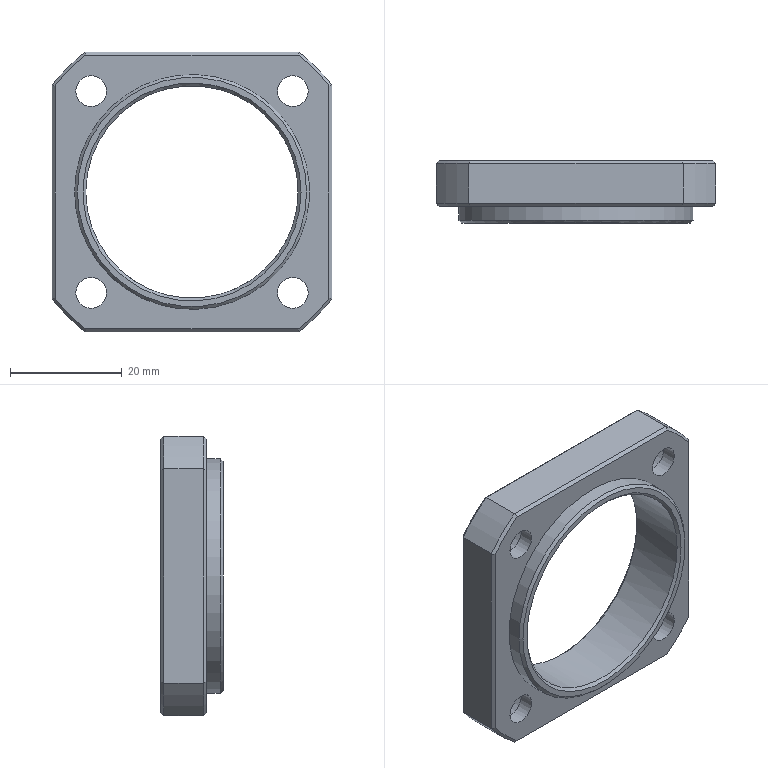Part | STEP file | BK-20_id1214_x_t | 1 solid | 44 faces | box 50 x 11.15 x 50 mm | volume 9475 mm3 | plane 19 | cylinder 14 | cone 11 | commonest cylinder face diameters 5.5 x4 9.5 x4 63 x4 38 x1 42 x1